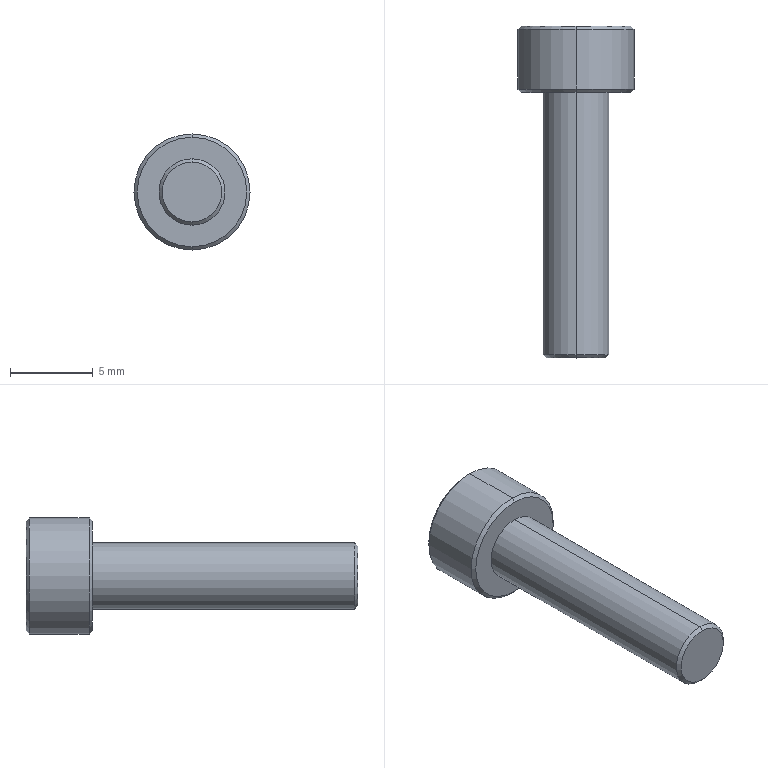Part | STEP file | Hex socket screw M4×16 | 1 solid | 33 faces | box 7 x 20 x 7 mm | volume 336.359 mm3 | cone 13 | plane 10 | spline 6 | cylinder 4 | commonest cylinder face diameters 4 x2 7 x2